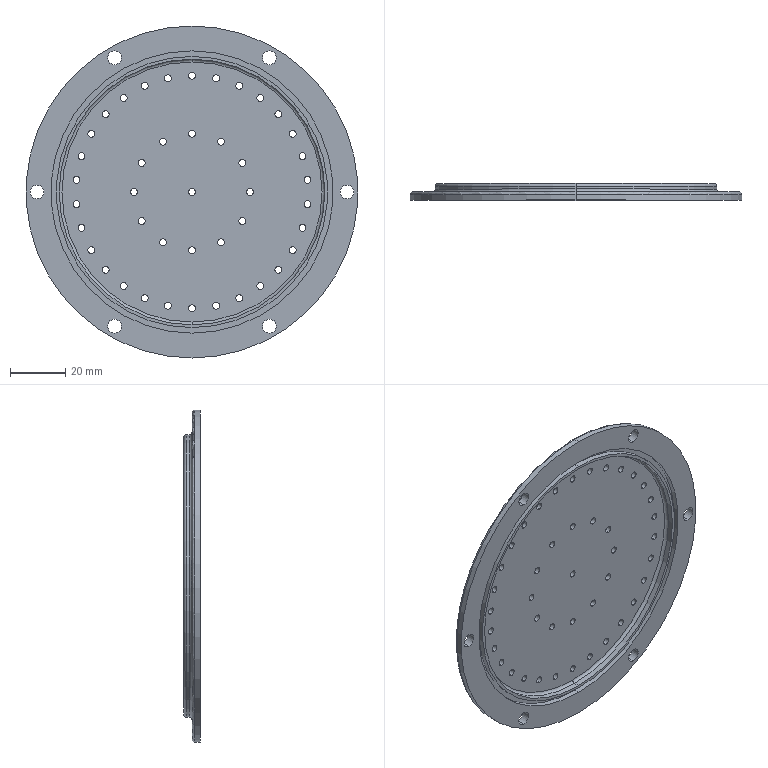Part | NX | features BREP 1 | 1 solid | 122 faces | box 120 x 6 x 120 mm | volume 34469 mm3 | cylinder 108 | torus 8 | plane 6 | commonest cylinder face diameters 2.5 x86 5 x12 102 x4 96 x2 98 x2 120 x2